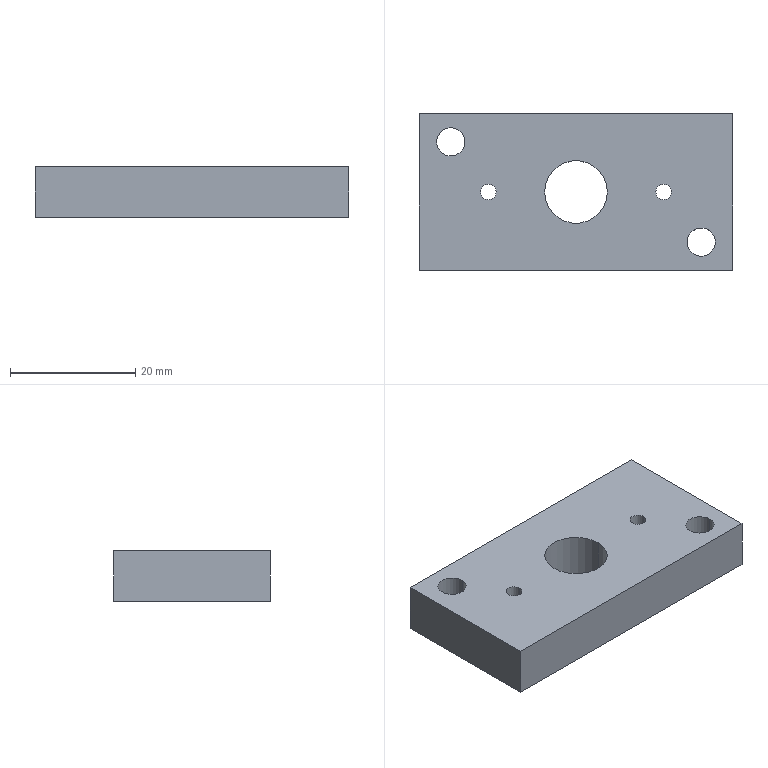Part | STEP file | positioning cylinder plate-1 | 1 solid | 16 faces | box 50 x 25 x 8 mm | volume 9039 mm3 | cylinder 10 | plane 6 | commonest cylinder face diameters 2.5 x4 4.5 x4 10 x2
STEP:
#1=CARTESIAN_POINT('',(0.,0.,0.));
#2=DIRECTION('',(0.,0.,1.));
#3=DIRECTION('',(1.,0.,0.));
#4=AXIS2_PLACEMENT_3D('',#1,#2,#3);
#5=CARTESIAN_POINT('',(-12.75,0.,0.));
#6=VERTEX_POINT('',#5);
#7=CARTESIAN_POINT('',(-12.75,0.,8.));
#8=VERTEX_POINT('',#7);
#9=CARTESIAN_POINT('',(-12.75,0.,8.));
#10=DIRECTION('',(0.,0.,1.));
#11=VECTOR('',#10,1.);
#12=LINE('',#9,#11);
#13=CARTESIAN_POINT('',(-14.,0.,8.));
#14=DIRECTION('',(0.,0.,1.));
#15=DIRECTION('',(1.,0.,0.));
#16=AXIS2_PLACEMENT_3D('',#13,#14,#15);
#17=CYLINDRICAL_SURFACE('',#16,1.25);
#18=CARTESIAN_POINT('',(6.283,0.));
#19=DIRECTION('',(0.,1.));
#20=VECTOR('',#19,1.);
#21=LINE('',#18,#20);
#22=(GEOMETRIC_REPRESENTATION_CONTEXT(2)PARAMETRIC_REPRESENTATION_CONTEXT()REPRESENTATION_CONTEXT('',''));
#23=DEFINITIONAL_REPRESENTATION('',(#21),#22);
#24=PCURVE('',#17,#23);
#25=CARTESIAN_POINT('',(-14.,0.,8.));
#26=DIRECTION('',(0.,0.,1.));
#27=DIRECTION('',(1.,0.,0.));
#28=AXIS2_PLACEMENT_3D('',#25,#26,#27);
#29=CYLINDRICAL_SURFACE('',#28,1.25);
#30=CARTESIAN_POINT('',(0.,0.));
#31=DIRECTION('',(0.,1.));
#32=VECTOR('',#31,1.);
#33=LINE('',#30,#32);
#34=(GEOMETRIC_REPRESENTATION_CONTEXT(2)PARAMETRIC_REPRESENTATION_CONTEXT()REPRESENTATION_CONTEXT('',''));
#35=DEFINITIONAL_REPRESENTATION('',(#33),#34);
#36=PCURVE('',#29,#35);
#37=SURFACE_CURVE('',#12,(#24,#36),.PCURVE_S1.);
#38=EDGE_CURVE('',#6,#8,#37,.T.);
#39=ORIENTED_EDGE('',*,*,#38,.T.);
#40=CARTESIAN_POINT('',(-15.25,0.,8.));
#41=VERTEX_POINT('',#40);
#42=CARTESIAN_POINT('',(-14.,0.,8.));
#43=DIRECTION('',(0.,0.,1.));
#44=DIRECTION('',(1.,0.,0.));
#45=AXIS2_PLACEMENT_3D('',#42,#43,#44);
#46=CIRCLE('',#45,1.25);
#47=CARTESIAN_POINT('',(0.,0.));
#48=DIRECTION('',(1.,0.));
#49=VECTOR('',#48,1.);
#50=LINE('',#47,#49);
#51=(GEOMETRIC_REPRESENTATION_CONTEXT(2)PARAMETRIC_REPRESENTATION_CONTEXT()REPRESENTATION_CONTEXT('',''));
#52=DEFINITIONAL_REPRESENTATION('',(#50),#51);
#53=PCURVE('',#17,#52);
#54=CARTESIAN_POINT('',(25.,-12.5,8.));
#55=DIRECTION('',(0.,0.,1.));
#56=DIRECTION('',(1.,0.,0.));
#57=AXIS2_PLACEMENT_3D('',#54,#55,#56);
#58=PLANE('',#57);
#59=CARTESIAN_POINT('',(-39.,12.5));
#60=DIRECTION('',(1.,0.));
#61=AXIS2_PLACEMENT_2D('',#59,#60);
#62=CIRCLE('',#61,1.25);
#63=(GEOMETRIC_REPRESENTATION_CONTEXT(2)PARAMETRIC_REPRESENTATION_CONTEXT()REPRESENTATION_CONTEXT('',''));
#64=DEFINITIONAL_REPRESENTATION('',(#62),#63);
#65=PCURVE('',#58,#64);
#66=SURFACE_CURVE('',#46,(#53,#65),.PCURVE_S1.);
#67=EDGE_CURVE('',#41,#8,#66,.T.);
#68=ORIENTED_EDGE('',*,*,#67,.F.);
#69=CARTESIAN_POINT('',(-15.25,0.,0.));
#70=VERTEX_POINT('',#69);
#71=CARTESIAN_POINT('',(-15.25,0.,8.));
#72=DIRECTION('',(0.,0.,1.));
#73=VECTOR('',#72,1.);
#74=LINE('',#71,#73);
#75=CARTESIAN_POINT('',(3.142,0.));
#76=DIRECTION('',(0.,1.));
#77=VECTOR('',#76,1.);
#78=LINE('',#75,#77);
#79=(GEOMETRIC_REPRESENTATION_CONTEXT(2)PARAMETRIC_REPRESENTATION_CONTEXT()REPRESENTATION_CONTEXT('',''));
#80=DEFINITIONAL_REPRESENTATION('',(#78),#79);
#81=PCURVE('',#17,#80);
#82=CARTESIAN_POINT('',(3.142,0.));
#83=DIRECTION('',(0.,1.));
#84=VECTOR('',#83,1.);
#85=LINE('',#82,#84);
#86=(GEOMETRIC_REPRESENTATION_CONTEXT(2)PARAMETRIC_REPRESENTATION_CONTEXT()REPRESENTATION_CONTEXT('',''));
#87=DEFINITIONAL_REPRESENTATION('',(#85),#86);
#88=PCURVE('',#29,#87);
#89=SURFACE_CURVE('',#74,(#81,#88),.PCURVE_S1.);
#90=EDGE_CURVE('',#70,#41,#89,.T.);
#91=ORIENTED_EDGE('',*,*,#90,.F.);
#92=CARTESIAN_POINT('',(-14.,0.,0.));
#93=DIRECTION('',(0.,0.,1.));
#94=DIRECTION('',(1.,0.,0.));
#95=AXIS2_PLACEMENT_3D('',#92,#93,#94);
#96=CIRCLE('',#95,1.25);
#97=CARTESIAN_POINT('',(0.,-8.));
#98=DIRECTION('',(1.,0.));
#99=VECTOR('',#98,1.);
#100=LINE('',#97,#99);
#101=(GEOMETRIC_REPRESENTATION_CONTEXT(2)PARAMETRIC_REPRESENTATION_CONTEXT()REPRESENTATION_CONTEXT('',''));
#102=DEFINITIONAL_REPRESENTATION('',(#100),#101);
#103=PCURVE('',#17,#102);
#104=CARTESIAN_POINT('',(25.,-12.5,0.));
#105=DIRECTION('',(0.,0.,1.));
#106=DIRECTION('',(1.,0.,0.));
#107=AXIS2_PLACEMENT_3D('',#104,#105,#106);
#108=PLANE('',#107);
#109=CARTESIAN_POINT('',(-39.,12.5));
#110=DIRECTION('',(1.,0.));
#111=AXIS2_PLACEMENT_2D('',#109,#110);
#112=CIRCLE('',#111,1.25);
#113=(GEOMETRIC_REPRESENTATION_CONTEXT(2)PARAMETRIC_REPRESENTATION_CONTEXT()REPRESENTATION_CONTEXT('',''));
#114=DEFINITIONAL_REPRESENTATION('',(#112),#113);
#115=PCURVE('',#108,#114);
#116=SURFACE_CURVE('',#96,(#103,#115),.PCURVE_S1.);
#117=EDGE_CURVE('',#70,#6,#116,.T.);
#118=ORIENTED_EDGE('',*,*,#117,.T.);
#119=EDGE_LOOP('',(#39,#68,#91,#118));
#120=FACE_BOUND('',#119,.F.);
#121=ADVANCED_FACE('',(#120),#17,.F.);
#122=CARTESIAN_POINT('',(15.25,0.,0.));
#123=VERTEX_POINT('',#122);
#124=CARTESIAN_POINT('',(15.25,0.,8.));
#125=VERTEX_POINT('',#124);
#126=CARTESIAN_POINT('',(15.25,0.,8.));
#127=DIRECTION('',(0.,0.,1.));
#128=VECTOR('',#127,1.);
#129=LINE('',#126,#128);
#130=CARTESIAN_POINT('',(14.,0.,8.));
#131=DIRECTION('',(0.,0.,1.));
#132=DIRECTION('',(1.,0.,0.));
#133=AXIS2_PLACEMENT_3D('',#130,#131,#132);
#134=CYLINDRICAL_SURFACE('',#133,1.25);
#135=CARTESIAN_POINT('',(6.283,0.));
#136=DIRECTION('',(0.,1.));
#137=VECTOR('',#136,1.);
#138=LINE('',#135,#137);
#139=(GEOMETRIC_REPRESENTATION_CONTEXT(2)PARAMETRIC_REPRESENTATION_CONTEXT()REPRESENTATION_CONTEXT('',''));
#140=DEFINITIONAL_REPRESENTATION('',(#138),#139);
#141=PCURVE('',#134,#140);
#142=CARTESIAN_POINT('',(14.,0.,8.));
#143=DIRECTION('',(0.,0.,1.));
#144=DIRECTION('',(1.,0.,0.));
#145=AXIS2_PLACEMENT_3D('',#142,#143,#144);
#146=CYLINDRICAL_SURFACE('',#145,1.25);
#147=CARTESIAN_POINT('',(0.,0.));
#148=DIRECTION('',(0.,1.));
#149=VECTOR('',#148,1.);
#150=LINE('',#147,#149);
#151=(GEOMETRIC_REPRESENTATION_CONTEXT(2)PARAMETRIC_REPRESENTATION_CONTEXT()REPRESENTATION_CONTEXT('',''));
#152=DEFINITIONAL_REPRESENTATION('',(#150),#151);
#153=PCURVE('',#146,#152);
#154=SURFACE_CURVE('',#129,(#141,#153),.PCURVE_S1.);
#155=EDGE_CURVE('',#123,#125,#154,.T.);
#156=ORIENTED_EDGE('',*,*,#155,.T.);
#157=CARTESIAN_POINT('',(12.75,0.,8.));
#158=VERTEX_POINT('',#157);
#159=CARTESIAN_POINT('',(14.,0.,8.));
#160=DIRECTION('',(0.,0.,1.));
#161=DIRECTION('',(1.,0.,0.));
#162=AXIS2_PLACEMENT_3D('',#159,#160,#161);
#163=CIRCLE('',#162,1.25);
#164=CARTESIAN_POINT('',(0.,0.));
#165=DIRECTION('',(1.,0.));
#166=VECTOR('',#165,1.);
#167=LINE('',#164,#166);
#168=(GEOMETRIC_REPRESENTATION_CONTEXT(2)PARAMETRIC_REPRESENTATION_CONTEXT()REPRESENTATION_CONTEXT('',''));
#169=DEFINITIONAL_REPRESENTATION('',(#167),#168);
#170=PCURVE('',#134,#169);
#171=CARTESIAN_POINT('',(-11.,12.5));
#172=DIRECTION('',(1.,0.));
#173=AXIS2_PLACEMENT_2D('',#171,#172);
#174=CIRCLE('',#173,1.25);
#175=(GEOMETRIC_REPRESENTATION_CONTEXT(2)PARAMETRIC_REPRESENTATION_CONTEXT()REPRESENTATION_CONTEXT('',''));
#176=DEFINITIONAL_REPRESENTATION('',(#174),#175);
#177=PCURVE('',#58,#176);
#178=SURFACE_CURVE('',#163,(#170,#177),.PCURVE_S1.);
#179=EDGE_CURVE('',#158,#125,#178,.T.);
#180=ORIENTED_EDGE('',*,*,#179,.F.);
#181=CARTESIAN_POINT('',(12.75,0.,0.));
#182=VERTEX_POINT('',#181);
#183=CARTESIAN_POINT('',(12.75,0.,8.));
#184=DIRECTION('',(0.,0.,1.));
#185=VECTOR('',#184,1.);
#186=LINE('',#183,#185);
#187=CARTESIAN_POINT('',(3.142,0.));
#188=DIRECTION('',(0.,1.));
#189=VECTOR('',#188,1.);
#190=LINE('',#187,#189);
#191=(GEOMETRIC_REPRESENTATION_CONTEXT(2)PARAMETRIC_REPRESENTATION_CONTEXT()REPRESENTATION_CONTEXT('',''));
#192=DEFINITIONAL_REPRESENTATION('',(#190),#191);
#193=PCURVE('',#134,#192);
#194=CARTESIAN_POINT('',(3.142,0.));
#195=DIRECTION('',(0.,1.));
#196=VECTOR('',#195,1.);
#197=LINE('',#194,#196);
#198=(GEOMETRIC_REPRESENTATION_CONTEXT(2)PARAMETRIC_REPRESENTATION_CONTEXT()REPRESENTATION_CONTEXT('',''));
#199=DEFINITIONAL_REPRESENTATION('',(#197),#198);
#200=PCURVE('',#146,#199);
#201=SURFACE_CURVE('',#186,(#193,#200),.PCURVE_S1.);
#202=EDGE_CURVE('',#182,#158,#201,.T.);
#203=ORIENTED_EDGE('',*,*,#202,.F.);
#204=CARTESIAN_POINT('',(14.,0.,0.));
#205=DIRECTION('',(0.,0.,1.));
#206=DIRECTION('',(1.,0.,0.));
#207=AXIS2_PLACEMENT_3D('',#204,#205,#206);
#208=CIRCLE('',#207,1.25);
#209=CARTESIAN_POINT('',(0.,-8.));
#210=DIRECTION('',(1.,0.));
#211=VECTOR('',#210,1.);
#212=LINE('',#209,#211);
#213=(GEOMETRIC_REPRESENTATION_CONTEXT(2)PARAMETRIC_REPRESENTATION_CONTEXT()REPRESENTATION_CONTEXT('',''));
#214=DEFINITIONAL_REPRESENTATION('',(#212),#213);
#215=PCURVE('',#134,#214);
#216=CARTESIAN_POINT('',(-11.,12.5));
#217=DIRECTION('',(1.,0.));
#218=AXIS2_PLACEMENT_2D('',#216,#217);
#219=CIRCLE('',#218,1.25);
#220=(GEOMETRIC_REPRESENTATION_CONTEXT(2)PARAMETRIC_REPRESENTATION_CONTEXT()REPRESENTATION_CONTEXT('',''));
#221=DEFINITIONAL_REPRESENTATION('',(#219),#220);
#222=PCURVE('',#108,#221);
#223=SURFACE_CURVE('',#208,(#215,#222),.PCURVE_S1.);
#224=EDGE_CURVE('',#182,#123,#223,.T.);
#225=ORIENTED_EDGE('',*,*,#224,.T.);
#226=EDGE_LOOP('',(#156,#180,#203,#225));
#227=FACE_BOUND('',#226,.F.);
#228=ADVANCED_FACE('',(#227),#134,.F.);
#229=CARTESIAN_POINT('',(-5.,0.,8.));
#230=VERTEX_POINT('',#229);
#231=CARTESIAN_POINT('',(-5.,0.,0.));
#232=VERTEX_POINT('',#231);
#233=CARTESIAN_POINT('',(-5.,0.,8.));
#234=DIRECTION('',(0.,0.,-1.));
#235=VECTOR('',#234,1.);
#236=LINE('',#233,#235);
#237=CARTESIAN_POINT('',(0.,0.,8.));
#238=DIRECTION('',(0.,0.,-1.));
#239=DIRECTION('',(-1.,0.,0.));
#240=AXIS2_PLACEMENT_3D('',#237,#238,#239);
#241=CYLINDRICAL_SURFACE('',#240,5.);
#242=CARTESIAN_POINT('',(6.283,0.));
#243=DIRECTION('',(0.,1.));
#244=VECTOR('',#243,1.);
#245=LINE('',#242,#244);
#246=(GEOMETRIC_REPRESENTATION_CONTEXT(2)PARAMETRIC_REPRESENTATION_CONTEXT()REPRESENTATION_CONTEXT('',''));
#247=DEFINITIONAL_REPRESENTATION('',(#245),#246);
#248=PCURVE('',#241,#247);
#249=CARTESIAN_POINT('',(0.,0.,8.));
#250=DIRECTION('',(0.,0.,-1.));
#251=DIRECTION('',(-1.,0.,0.));
#252=AXIS2_PLACEMENT_3D('',#249,#250,#251);
#253=CYLINDRICAL_SURFACE('',#252,5.);
#254=CARTESIAN_POINT('',(0.,0.));
#255=DIRECTION('',(0.,1.));
#256=VECTOR('',#255,1.);
#257=LINE('',#254,#256);
#258=(GEOMETRIC_REPRESENTATION_CONTEXT(2)PARAMETRIC_REPRESENTATION_CONTEXT()REPRESENTATION_CONTEXT('',''));
#259=DEFINITIONAL_REPRESENTATION('',(#257),#258);
#260=PCURVE('',#253,#259);
#261=SURFACE_CURVE('',#236,(#248,#260),.PCURVE_S1.);
#262=EDGE_CURVE('',#230,#232,#261,.T.);
#263=ORIENTED_EDGE('',*,*,#262,.T.);
#264=CARTESIAN_POINT('',(5.,0.,0.));
#265=VERTEX_POINT('',#264);
#266=CARTESIAN_POINT('',(0.,0.,0.));
#267=DIRECTION('',(0.,0.,1.));
#268=DIRECTION('',(1.,0.,0.));
#269=AXIS2_PLACEMENT_3D('',#266,#267,#268);
#270=CIRCLE('',#269,5.);
#271=CARTESIAN_POINT('',(9.425,8.));
#272=DIRECTION('',(-1.,0.));
#273=VECTOR('',#272,1.);
#274=LINE('',#271,#273);
#275=(GEOMETRIC_REPRESENTATION_CONTEXT(2)PARAMETRIC_REPRESENTATION_CONTEXT()REPRESENTATION_CONTEXT('',''));
#276=DEFINITIONAL_REPRESENTATION('',(#274),#275);
#277=PCURVE('',#241,#276);
#278=CARTESIAN_POINT('',(-25.,12.5));
#279=DIRECTION('',(1.,0.));
#280=AXIS2_PLACEMENT_2D('',#278,#279);
#281=CIRCLE('',#280,5.);
#282=(GEOMETRIC_REPRESENTATION_CONTEXT(2)PARAMETRIC_REPRESENTATION_CONTEXT()REPRESENTATION_CONTEXT('',''));
#283=DEFINITIONAL_REPRESENTATION('',(#281),#282);
#284=PCURVE('',#108,#283);
#285=SURFACE_CURVE('',#270,(#277,#284),.PCURVE_S1.);
#286=EDGE_CURVE('',#232,#265,#285,.T.);
#287=ORIENTED_EDGE('',*,*,#286,.T.);
#288=CARTESIAN_POINT('',(5.,0.,8.));
#289=VERTEX_POINT('',#288);
#290=CARTESIAN_POINT('',(5.,0.,8.));
#291=DIRECTION('',(0.,0.,-1.));
#292=VECTOR('',#291,1.);
#293=LINE('',#290,#292);
#294=CARTESIAN_POINT('',(3.142,0.));
#295=DIRECTION('',(0.,1.));
#296=VECTOR('',#295,1.);
#297=LINE('',#294,#296);
#298=(GEOMETRIC_REPRESENTATION_CONTEXT(2)PARAMETRIC_REPRESENTATION_CONTEXT()REPRESENTATION_CONTEXT('',''));
#299=DEFINITIONAL_REPRESENTATION('',(#297),#298);
#300=PCURVE('',#241,#299);
#301=CARTESIAN_POINT('',(3.142,0.));
#302=DIRECTION('',(0.,1.));
#303=VECTOR('',#302,1.);
#304=LINE('',#301,#303);
#305=(GEOMETRIC_REPRESENTATION_CONTEXT(2)PARAMETRIC_REPRESENTATION_CONTEXT()REPRESENTATION_CONTEXT('',''));
#306=DEFINITIONAL_REPRESENTATION('',(#304),#305);
#307=PCURVE('',#253,#306);
#308=SURFACE_CURVE('',#293,(#300,#307),.PCURVE_S1.);
#309=EDGE_CURVE('',#289,#265,#308,.T.);
#310=ORIENTED_EDGE('',*,*,#309,.F.);
#311=CARTESIAN_POINT('',(0.,0.,8.));
#312=DIRECTION('',(0.,0.,1.));
#313=DIRECTION('',(1.,0.,0.));
#314=AXIS2_PLACEMENT_3D('',#311,#312,#313);
#315=CIRCLE('',#314,5.);
#316=CARTESIAN_POINT('',(9.425,0.));
#317=DIRECTION('',(-1.,0.));
#318=VECTOR('',#317,1.);
#319=LINE('',#316,#318);
#320=(GEOMETRIC_REPRESENTATION_CONTEXT(2)PARAMETRIC_REPRESENTATION_CONTEXT()REPRESENTATION_CONTEXT('',''));
#321=DEFINITIONAL_REPRESENTATION('',(#319),#320);
#322=PCURVE('',#241,#321);
#323=CARTESIAN_POINT('',(-25.,12.5));
#324=DIRECTION('',(1.,0.));
#325=AXIS2_PLACEMENT_2D('',#323,#324);
#326=CIRCLE('',#325,5.);
#327=(GEOMETRIC_REPRESENTATION_CONTEXT(2)PARAMETRIC_REPRESENTATION_CONTEXT()REPRESENTATION_CONTEXT('',''));
#328=DEFINITIONAL_REPRESENTATION('',(#326),#327);
#329=PCURVE('',#58,#328);
#330=SURFACE_CURVE('',#315,(#322,#329),.PCURVE_S1.);
#331=EDGE_CURVE('',#230,#289,#330,.T.);
#332=ORIENTED_EDGE('',*,*,#331,.F.);
#333=EDGE_LOOP('',(#263,#287,#310,#332));
#334=FACE_BOUND('',#333,.F.);
#335=ADVANCED_FACE('',(#334),#241,.F.);
#336=CARTESIAN_POINT('',(-22.25,8.,8.));
#337=VERTEX_POINT('',#336);
#338=CARTESIAN_POINT('',(-22.25,8.,0.));
#339=VERTEX_POINT('',#338);
#340=CARTESIAN_POINT('',(-22.25,8.,8.));
#341=DIRECTION('',(0.,0.,-1.));
#342=VECTOR('',#341,1.);
#343=LINE('',#340,#342);
#344=CARTESIAN_POINT('',(-20.,8.,8.));
#345=DIRECTION('',(0.,0.,-1.));
#346=DIRECTION('',(-1.,0.,0.));
#347=AXIS2_PLACEMENT_3D('',#344,#345,#346);
#348=CYLINDRICAL_SURFACE('',#347,2.25);
#349=CARTESIAN_POINT('',(6.283,0.));
#350=DIRECTION('',(0.,1.));
#351=VECTOR('',#350,1.);
#352=LINE('',#349,#351);
#353=(GEOMETRIC_REPRESENTATION_CONTEXT(2)PARAMETRIC_REPRESENTATION_CONTEXT()REPRESENTATION_CONTEXT('',''));
#354=DEFINITIONAL_REPRESENTATION('',(#352),#353);
#355=PCURVE('',#348,#354);
#356=CARTESIAN_POINT('',(-20.,8.,8.));
#357=DIRECTION('',(0.,0.,-1.));
#358=DIRECTION('',(-1.,0.,0.));
#359=AXIS2_PLACEMENT_3D('',#356,#357,#358);
#360=CYLINDRICAL_SURFACE('',#359,2.25);
#361=CARTESIAN_POINT('',(0.,0.));
#362=DIRECTION('',(0.,1.));
#363=VECTOR('',#362,1.);
#364=LINE('',#361,#363);
#365=(GEOMETRIC_REPRESENTATION_CONTEXT(2)PARAMETRIC_REPRESENTATION_CONTEXT()REPRESENTATION_CONTEXT('',''));
#366=DEFINITIONAL_REPRESENTATION('',(#364),#365);
#367=PCURVE('',#360,#366);
#368=SURFACE_CURVE('',#343,(#355,#367),.PCURVE_S1.);
#369=EDGE_CURVE('',#337,#339,#368,.T.);
#370=ORIENTED_EDGE('',*,*,#369,.T.);
#371=CARTESIAN_POINT('',(-17.75,8.,0.));
#372=VERTEX_POINT('',#371);
#373=CARTESIAN_POINT('',(-20.,8.,0.));
#374=DIRECTION('',(0.,0.,1.));
#375=DIRECTION('',(1.,0.,0.));
#376=AXIS2_PLACEMENT_3D('',#373,#374,#375);
#377=CIRCLE('',#376,2.25);
#378=CARTESIAN_POINT('',(9.425,8.));
#379=DIRECTION('',(-1.,0.));
#380=VECTOR('',#379,1.);
#381=LINE('',#378,#380);
#382=(GEOMETRIC_REPRESENTATION_CONTEXT(2)PARAMETRIC_REPRESENTATION_CONTEXT()REPRESENTATION_CONTEXT('',''));
#383=DEFINITIONAL_REPRESENTATION('',(#381),#382);
#384=PCURVE('',#348,#383);
#385=CARTESIAN_POINT('',(-45.,20.5));
#386=DIRECTION('',(1.,0.));
#387=AXIS2_PLACEMENT_2D('',#385,#386);
#388=CIRCLE('',#387,2.25);
#389=(GEOMETRIC_REPRESENTATION_CONTEXT(2)PARAMETRIC_REPRESENTATION_CONTEXT()REPRESENTATION_CONTEXT('',''));
#390=DEFINITIONAL_REPRESENTATION('',(#388),#389);
#391=PCURVE('',#108,#390);
#392=SURFACE_CURVE('',#377,(#384,#391),.PCURVE_S1.);
#393=EDGE_CURVE('',#339,#372,#392,.T.);
#394=ORIENTED_EDGE('',*,*,#393,.T.);
#395=CARTESIAN_POINT('',(-17.75,8.,8.));
#396=VERTEX_POINT('',#395);
#397=CARTESIAN_POINT('',(-17.75,8.,8.));
#398=DIRECTION('',(0.,0.,-1.));
#399=VECTOR('',#398,1.);
#400=LINE('',#397,#399);
#401=CARTESIAN_POINT('',(3.142,0.));
#402=DIRECTION('',(0.,1.));
#403=VECTOR('',#402,1.);
#404=LINE('',#401,#403);
#405=(GEOMETRIC_REPRESENTATION_CONTEXT(2)PARAMETRIC_REPRESENTATION_CONTEXT()REPRESENTATION_CONTEXT('',''));
#406=DEFINITIONAL_REPRESENTATION('',(#404),#405);
#407=PCURVE('',#348,#406);
#408=CARTESIAN_POINT('',(3.142,0.));
#409=DIRECTION('',(0.,1.));
#410=VECTOR('',#409,1.);
#411=LINE('',#408,#410);
#412=(GEOMETRIC_REPRESENTATION_CONTEXT(2)PARAMETRIC_REPRESENTATION_CONTEXT()REPRESENTATION_CONTEXT('',''));
#413=DEFINITIONAL_REPRESENTATION('',(#411),#412);
#414=PCURVE('',#360,#413);
#415=SURFACE_CURVE('',#400,(#407,#414),.PCURVE_S1.);
#416=EDGE_CURVE('',#396,#372,#415,.T.);
#417=ORIENTED_EDGE('',*,*,#416,.F.);
#418=CARTESIAN_POINT('',(-20.,8.,8.));
#419=DIRECTION('',(0.,0.,1.));
#420=DIRECTION('',(1.,0.,0.));
#421=AXIS2_PLACEMENT_3D('',#418,#419,#420);
#422=CIRCLE('',#421,2.25);
#423=CARTESIAN_POINT('',(9.425,0.));
#424=DIRECTION('',(-1.,0.));
#425=VECTOR('',#424,1.);
#426=LINE('',#423,#425);
#427=(GEOMETRIC_REPRESENTATION_CONTEXT(2)PARAMETRIC_REPRESENTATION_CONTEXT()REPRESENTATION_CONTEXT('',''));
#428=DEFINITIONAL_REPRESENTATION('',(#426),#427);
#429=PCURVE('',#348,#428);
#430=CARTESIAN_POINT('',(-45.,20.5));
#431=DIRECTION('',(1.,0.));
#432=AXIS2_PLACEMENT_2D('',#430,#431);
#433=CIRCLE('',#432,2.25);
#434=(GEOMETRIC_REPRESENTATION_CONTEXT(2)PARAMETRIC_REPRESENTATION_CONTEXT()REPRESENTATION_CONTEXT('',''));
#435=DEFINITIONAL_REPRESENTATION('',(#433),#434);
#436=PCURVE('',#58,#435);
#437=SURFACE_CURVE('',#422,(#429,#436),.PCURVE_S1.);
#438=EDGE_CURVE('',#337,#396,#437,.T.);
#439=ORIENTED_EDGE('',*,*,#438,.F.);
#440=EDGE_LOOP('',(#370,#394,#417,#439));
#441=FACE_BOUND('',#440,.F.);
#442=ADVANCED_FACE('',(#441),#348,.F.);
#443=CARTESIAN_POINT('',(17.75,-8.,8.));
#444=VERTEX_POINT('',#443);
#445=CARTESIAN_POINT('',(17.75,-8.,0.));
#446=VERTEX_POINT('',#445);
#447=CARTESIAN_POINT('',(17.75,-8.,8.));
#448=DIRECTION('',(0.,0.,-1.));
#449=VECTOR('',#448,1.);
#450=LINE('',#447,#449);
#451=CARTESIAN_POINT('',(20.,-8.,8.));
#452=DIRECTION('',(0.,0.,-1.));
#453=DIRECTION('',(-1.,0.,0.));
#454=AXIS2_PLACEMENT_3D('',#451,#452,#453);
#455=CYLINDRICAL_SURFACE('',#454,2.25);
#456=CARTESIAN_POINT('',(6.283,0.));
#457=DIRECTION('',(0.,1.));
#458=VECTOR('',#457,1.);
#459=LINE('',#456,#458);
#460=(GEOMETRIC_REPRESENTATION_CONTEXT(2)PARAMETRIC_REPRESENTATION_CONTEXT()REPRESENTATION_CONTEXT('',''));
#461=DEFINITIONAL_REPRESENTATION('',(#459),#460);
#462=PCURVE('',#455,#461);
#463=CARTESIAN_POINT('',(20.,-8.,8.));
#464=DIRECTION('',(0.,0.,-1.));
#465=DIRECTION('',(-1.,0.,0.));
#466=AXIS2_PLACEMENT_3D('',#463,#464,#465);
#467=CYLINDRICAL_SURFACE('',#466,2.25);
#468=CARTESIAN_POINT('',(0.,0.));
#469=DIRECTION('',(0.,1.));
#470=VECTOR('',#469,1.);
#471=LINE('',#468,#470);
#472=(GEOMETRIC_REPRESENTATION_CONTEXT(2)PARAMETRIC_REPRESENTATION_CONTEXT()REPRESENTATION_CONTEXT('',''));
#473=DEFINITIONAL_REPRESENTATION('',(#471),#472);
#474=PCURVE('',#467,#473);
#475=SURFACE_CURVE('',#450,(#462,#474),.PCURVE_S1.);
#476=EDGE_CURVE('',#444,#446,#475,.T.);
#477=ORIENTED_EDGE('',*,*,#476,.T.);
#478=CARTESIAN_POINT('',(22.25,-8.,0.));
#479=VERTEX_POINT('',#478);
#480=CARTESIAN_POINT('',(20.,-8.,0.));
#481=DIRECTION('',(0.,0.,1.));
#482=DIRECTION('',(1.,0.,0.));
#483=AXIS2_PLACEMENT_3D('',#480,#481,#482);
#484=CIRCLE('',#483,2.25);
#485=CARTESIAN_POINT('',(9.425,8.));
#486=DIRECTION('',(-1.,0.));
#487=VECTOR('',#486,1.);
#488=LINE('',#485,#487);
#489=(GEOMETRIC_REPRESENTATION_CONTEXT(2)PARAMETRIC_REPRESENTATION_CONTEXT()REPRESENTATION_CONTEXT('',''));
#490=DEFINITIONAL_REPRESENTATION('',(#488),#489);
#491=PCURVE('',#455,#490);
#492=CARTESIAN_POINT('',(-5.,4.5));
#493=DIRECTION('',(1.,0.));
#494=AXIS2_PLACEMENT_2D('',#492,#493);
#495=CIRCLE('',#494,2.25);
#496=(GEOMETRIC_REPRESENTATION_CONTEXT(2)PARAMETRIC_REPRESENTATION_CONTEXT()REPRESENTATION_CONTEXT('',''));
#497=DEFINITIONAL_REPRESENTATION('',(#495),#496);
#498=PCURVE('',#108,#497);
#499=SURFACE_CURVE('',#484,(#491,#498),.PCURVE_S1.);
#500=EDGE_CURVE('',#446,#479,#499,.T.);
#501=ORIENTED_EDGE('',*,*,#500,.T.);
#502=CARTESIAN_POINT('',(22.25,-8.,8.));
#503=VERTEX_POINT('',#502);
#504=CARTESIAN_POINT('',(22.25,-8.,8.));
#505=DIRECTION('',(0.,0.,-1.));
#506=VECTOR('',#505,1.);
#507=LINE('',#504,#506);
#508=CARTESIAN_POINT('',(3.142,0.));
#509=DIRECTION('',(0.,1.));
#510=VECTOR('',#509,1.);
#511=LINE('',#508,#510);
#512=(GEOMETRIC_REPRESENTATION_CONTEXT(2)PARAMETRIC_REPRESENTATION_CONTEXT()REPRESENTATION_CONTEXT('',''));
#513=DEFINITIONAL_REPRESENTATION('',(#511),#512);
#514=PCURVE('',#455,#513);
#515=CARTESIAN_POINT('',(3.142,0.));
#516=DIRECTION('',(0.,1.));
#517=VECTOR('',#516,1.);
#518=LINE('',#515,#517);
#519=(GEOMETRIC_REPRESENTATION_CONTEXT(2)PARAMETRIC_REPRESENTATION_CONTEXT()REPRESENTATION_CONTEXT('',''));
#520=DEFINITIONAL_REPRESENTATION('',(#518),#519);
#521=PCURVE('',#467,#520);
#522=SURFACE_CURVE('',#507,(#514,#521),.PCURVE_S1.);
#523=EDGE_CURVE('',#503,#479,#522,.T.);
#524=ORIENTED_EDGE('',*,*,#523,.F.);
#525=CARTESIAN_POINT('',(20.,-8.,8.));
#526=DIRECTION('',(0.,0.,1.));
#527=DIRECTION('',(1.,0.,0.));
#528=AXIS2_PLACEMENT_3D('',#525,#526,#527);
#529=CIRCLE('',#528,2.25);
#530=CARTESIAN_POINT('',(9.425,0.));
#531=DIRECTION('',(-1.,0.));
#532=VECTOR('',#531,1.);
#533=LINE('',#530,#532);
#534=(GEOMETRIC_REPRESENTATION_CONTEXT(2)PARAMETRIC_REPRESENTATION_CONTEXT()REPRESENTATION_CONTEXT('',''));
#535=DEFINITIONAL_REPRESENTATION('',(#533),#534);
#536=PCURVE('',#455,#535);
#537=CARTESIAN_POINT('',(-5.,4.5));
#538=DIRECTION('',(1.,0.));
#539=AXIS2_PLACEMENT_2D('',#537,#538);
#540=CIRCLE('',#539,2.25);
#541=(GEOMETRIC_REPRESENTATION_CONTEXT(2)PARAMETRIC_REPRESENTATION_CONTEXT()REPRESENTATION_CONTEXT('',''));
#542=DEFINITIONAL_REPRESENTATION('',(#540),#541);
#543=PCURVE('',#58,#542);
#544=SURFACE_CURVE('',#529,(#536,#543),.PCURVE_S1.);
#545=EDGE_CURVE('',#444,#503,#544,.T.);
#546=ORIENTED_EDGE('',*,*,#545,.F.);
#547=EDGE_LOOP('',(#477,#501,#524,#546));
#548=FACE_BOUND('',#547,.F.);
#549=ADVANCED_FACE('',(#548),#455,.F.);
#550=CARTESIAN_POINT('',(-14.,0.,8.));
#551=DIRECTION('',(0.,0.,1.));
#552=DIRECTION('',(1.,0.,0.));
#553=AXIS2_PLACEMENT_3D('',#550,#551,#552);
#554=CIRCLE('',#553,1.25);
#555=CARTESIAN_POINT('',(-39.,12.5));
#556=DIRECTION('',(1.,0.));
#557=AXIS2_PLACEMENT_2D('',#555,#556);
#558=CIRCLE('',#557,1.25);
#559=(GEOMETRIC_REPRESENTATION_CONTEXT(2)PARAMETRIC_REPRESENTATION_CONTEXT()REPRESENTATION_CONTEXT('',''));
#560=DEFINITIONAL_REPRESENTATION('',(#558),#559);
#561=PCURVE('',#58,#560);
#562=CARTESIAN_POINT('',(0.,0.));
#563=DIRECTION('',(1.,0.));
#564=VECTOR('',#563,1.);
#565=LINE('',#562,#564);
#566=(GEOMETRIC_REPRESENTATION_CONTEXT(2)PARAMETRIC_REPRESENTATION_CONTEXT()REPRESENTATION_CONTEXT('',''));
#567=DEFINITIONAL_REPRESENTATION('',(#565),#566);
#568=PCURVE('',#29,#567);
#569=SURFACE_CURVE('',#554,(#561,#568),.PCURVE_S1.);
#570=EDGE_CURVE('',#8,#41,#569,.T.);
#571=ORIENTED_EDGE('',*,*,#570,.F.);
#572=ORIENTED_EDGE('',*,*,#67,.F.);
#573=EDGE_LOOP('',(#571,#572));
#574=FACE_BOUND('',#573,.T.);
#575=CARTESIAN_POINT('',(14.,0.,8.));
#576=DIRECTION('',(0.,0.,1.));
#577=DIRECTION('',(1.,0.,0.));
#578=AXIS2_PLACEMENT_3D('',#575,#576,#577);
#579=CIRCLE('',#578,1.25);
#580=CARTESIAN_POINT('',(-11.,12.5));
#581=DIRECTION('',(1.,0.));
#582=AXIS2_PLACEMENT_2D('',#580,#581);
#583=CIRCLE('',#582,1.25);
#584=(GEOMETRIC_REPRESENTATION_CONTEXT(2)PARAMETRIC_REPRESENTATION_CONTEXT()REPRESENTATION_CONTEXT('',''));
#585=DEFINITIONAL_REPRESENTATION('',(#583),#584);
#586=PCURVE('',#58,#585);
#587=CARTESIAN_POINT('',(0.,0.));
#588=DIRECTION('',(1.,0.));
#589=VECTOR('',#588,1.);
#590=LINE('',#587,#589);
#591=(GEOMETRIC_REPRESENTATION_CONTEXT(2)PARAMETRIC_REPRESENTATION_CONTEXT()REPRESENTATION_CONTEXT('',''));
#592=DEFINITIONAL_REPRESENTATION('',(#590),#591);
#593=PCURVE('',#146,#592);
#594=SURFACE_CURVE('',#579,(#586,#593),.PCURVE_S1.);
#595=EDGE_CURVE('',#125,#158,#594,.T.);
#596=ORIENTED_EDGE('',*,*,#595,.F.);
#597=ORIENTED_EDGE('',*,*,#179,.F.);
#598=EDGE_LOOP('',(#596,#597));
#599=FACE_BOUND('',#598,.T.);
#600=ORIENTED_EDGE('',*,*,#438,.F.);
#601=CARTESIAN_POINT('',(-20.,8.,8.));
#602=DIRECTION('',(0.,0.,1.));
#603=DIRECTION('',(1.,0.,0.));
#604=AXIS2_PLACEMENT_3D('',#601,#602,#603);
#605=CIRCLE('',#604,2.25);
#606=CARTESIAN_POINT('',(-45.,20.5));
#607=DIRECTION('',(1.,0.));
#608=AXIS2_PLACEMENT_2D('',#606,#607);
#609=CIRCLE('',#608,2.25);
#610=(GEOMETRIC_REPRESENTATION_CONTEXT(2)PARAMETRIC_REPRESENTATION_CONTEXT()REPRESENTATION_CONTEXT('',''));
#611=DEFINITIONAL_REPRESENTATION('',(#609),#610);
#612=PCURVE('',#58,#611);
#613=CARTESIAN_POINT('',(3.142,0.));
#614=DIRECTION('',(-1.,0.));
#615=VECTOR('',#614,1.);
#616=LINE('',#613,#615);
#617=(GEOMETRIC_REPRESENTATION_CONTEXT(2)PARAMETRIC_REPRESENTATION_CONTEXT()REPRESENTATION_CONTEXT('',''));
#618=DEFINITIONAL_REPRESENTATION('',(#616),#617);
#619=PCURVE('',#360,#618);
#620=SURFACE_CURVE('',#605,(#612,#619),.PCURVE_S1.);
#621=EDGE_CURVE('',#396,#337,#620,.T.);
#622=ORIENTED_EDGE('',*,*,#621,.F.);
#623=EDGE_LOOP('',(#600,#622));
#624=FACE_BOUND('',#623,.T.);
#625=CARTESIAN_POINT('',(25.,-12.5,8.));
#626=VERTEX_POINT('',#625);
#627=CARTESIAN_POINT('',(25.,12.5,8.));
#628=VERTEX_POINT('',#627);
#629=CARTESIAN_POINT('',(25.,12.5,8.));
#630=DIRECTION('',(0.,1.,0.));
#631=VECTOR('',#630,1.);
#632=LINE('',#629,#631);
#633=CARTESIAN_POINT('',(0.,25.));
#634=DIRECTION('',(0.,1.));
#635=VECTOR('',#634,1.);
#636=LINE('',#633,#635);
#637=(GEOMETRIC_REPRESENTATION_CONTEXT(2)PARAMETRIC_REPRESENTATION_CONTEXT()REPRESENTATION_CONTEXT('',''));
#638=DEFINITIONAL_REPRESENTATION('',(#636),#637);
#639=PCURVE('',#58,#638);
#640=CARTESIAN_POINT('',(25.,12.5,8.));
#641=DIRECTION('',(-1.,0.,0.));
#642=DIRECTION('',(0.,-1.,0.));
#643=AXIS2_PLACEMENT_3D('',#640,#641,#642);
#644=PLANE('',#643);
#645=CARTESIAN_POINT('',(0.,0.));
#646=DIRECTION('',(-1.,0.));
#647=VECTOR('',#646,1.);
#648=LINE('',#645,#647);
#649=(GEOMETRIC_REPRESENTATION_CONTEXT(2)PARAMETRIC_REPRESENTATION_CONTEXT()REPRESENTATION_CONTEXT('',''));
#650=DEFINITIONAL_REPRESENTATION('',(#648),#649);
#651=PCURVE('',#644,#650);
#652=SURFACE_CURVE('',#632,(#639,#651),.PCURVE_S1.);
#653=EDGE_CURVE('',#626,#628,#652,.T.);
#654=ORIENTED_EDGE('',*,*,#653,.T.);
#655=CARTESIAN_POINT('',(-25.,12.5,8.));
#656=VERTEX_POINT('',#655);
#657=CARTESIAN_POINT('',(-25.,12.5,8.));
#658=DIRECTION('',(-1.,0.,0.));
#659=VECTOR('',#658,1.);
#660=LINE('',#657,#659);
#661=CARTESIAN_POINT('',(-50.,25.));
#662=DIRECTION('',(-1.,0.));
#663=VECTOR('',#662,1.);
#664=LINE('',#661,#663);
#665=(GEOMETRIC_REPRESENTATION_CONTEXT(2)PARAMETRIC_REPRESENTATION_CONTEXT()REPRESENTATION_CONTEXT('',''));
#666=DEFINITIONAL_REPRESENTATION('',(#664),#665);
#667=PCURVE('',#58,#666);
#668=CARTESIAN_POINT('',(-25.,12.5,8.));
#669=DIRECTION('',(0.,-1.,0.));
#670=DIRECTION('',(0.,0.,-1.));
#671=AXIS2_PLACEMENT_3D('',#668,#669,#670);
#672=PLANE('',#671);
#673=CARTESIAN_POINT('',(0.,0.));
#674=DIRECTION('',(0.,-1.));
#675=VECTOR('',#674,1.);
#676=LINE('',#673,#675);
#677=(GEOMETRIC_REPRESENTATION_CONTEXT(2)PARAMETRIC_REPRESENTATION_CONTEXT()REPRESENTATION_CONTEXT('',''));
#678=DEFINITIONAL_REPRESENTATION('',(#676),#677);
#679=PCURVE('',#672,#678);
#680=SURFACE_CURVE('',#660,(#667,#679),.PCURVE_S1.);
#681=EDGE_CURVE('',#628,#656,#680,.T.);
#682=ORIENTED_EDGE('',*,*,#681,.T.);
#683=CARTESIAN_POINT('',(-25.,-12.5,8.));
#684=VERTEX_POINT('',#683);
#685=CARTESIAN_POINT('',(-25.,12.5,8.));
#686=DIRECTION('',(0.,-1.,0.));
#687=VECTOR('',#686,1.);
#688=LINE('',#685,#687);
#689=CARTESIAN_POINT('',(-50.,25.));
#690=DIRECTION('',(0.,-1.));
#691=VECTOR('',#690,1.);
#692=LINE('',#689,#691);
#693=(GEOMETRIC_REPRESENTATION_CONTEXT(2)PARAMETRIC_REPRESENTATION_CONTEXT()REPRESENTATION_CONTEXT('',''));
#694=DEFINITIONAL_REPRESENTATION('',(#692),#693);
#695=PCURVE('',#58,#694);
#696=CARTESIAN_POINT('',(-25.,12.5,8.));
#697=DIRECTION('',(1.,0.,0.));
#698=DIRECTION('',(0.,1.,0.));
#699=AXIS2_PLACEMENT_3D('',#696,#697,#698);
#700=PLANE('',#699);
#701=CARTESIAN_POINT('',(0.,0.));
#702=DIRECTION('',(-1.,0.));
#703=VECTOR('',#702,1.);
#704=LINE('',#701,#703);
#705=(GEOMETRIC_REPRESENTATION_CONTEXT(2)PARAMETRIC_REPRESENTATION_CONTEXT()REPRESENTATION_CONTEXT('',''));
#706=DEFINITIONAL_REPRESENTATION('',(#704),#705);
#707=PCURVE('',#700,#706);
#708=SURFACE_CURVE('',#688,(#695,#707),.PCURVE_S1.);
#709=EDGE_CURVE('',#656,#684,#708,.T.);
#710=ORIENTED_EDGE('',*,*,#709,.T.);
#711=CARTESIAN_POINT('',(-25.,-12.5,8.));
#712=DIRECTION('',(1.,0.,0.));
#713=VECTOR('',#712,1.);
#714=LINE('',#711,#713);
#715=CARTESIAN_POINT('',(-50.,0.));
#716=DIRECTION('',(1.,0.));
#717=VECTOR('',#716,1.);
#718=LINE('',#715,#717);
#719=(GEOMETRIC_REPRESENTATION_CONTEXT(2)PARAMETRIC_REPRESENTATION_CONTEXT()REPRESENTATION_CONTEXT('',''));
#720=DEFINITIONAL_REPRESENTATION('',(#718),#719);
#721=PCURVE('',#58,#720);
#722=CARTESIAN_POINT('',(-25.,-12.5,8.));
#723=DIRECTION('',(0.,1.,0.));
#724=DIRECTION('',(0.,0.,1.));
#725=AXIS2_PLACEMENT_3D('',#722,#723,#724);
#726=PLANE('',#725);
#727=CARTESIAN_POINT('',(0.,0.));
#728=DIRECTION('',(0.,1.));
#729=VECTOR('',#728,1.);
#730=LINE('',#727,#729);
#731=(GEOMETRIC_REPRESENTATION_CONTEXT(2)PARAMETRIC_REPRESENTATION_CONTEXT()REPRESENTATION_CONTEXT('',''));
#732=DEFINITIONAL_REPRESENTATION('',(#730),#731);
#733=PCURVE('',#726,#732);
#734=SURFACE_CURVE('',#714,(#721,#733),.PCURVE_S1.);
#735=EDGE_CURVE('',#684,#626,#734,.T.);
#736=ORIENTED_EDGE('',*,*,#735,.T.);
#737=EDGE_LOOP('',(#654,#682,#710,#736));
#738=FACE_BOUND('',#737,.T.);
#739=ORIENTED_EDGE('',*,*,#545,.F.);
#740=CARTESIAN_POINT('',(20.,-8.,8.));
#741=DIRECTION('',(0.,0.,1.));
#742=DIRECTION('',(1.,0.,0.));
#743=AXIS2_PLACEMENT_3D('',#740,#741,#742);
#744=CIRCLE('',#743,2.25);
#745=CARTESIAN_POINT('',(-5.,4.5));
#746=DIRECTION('',(1.,0.));
#747=AXIS2_PLACEMENT_2D('',#745,#746);
#748=CIRCLE('',#747,2.25);
#749=(GEOMETRIC_REPRESENTATION_CONTEXT(2)PARAMETRIC_REPRESENTATION_CONTEXT()REPRESENTATION_CONTEXT('',''));
#750=DEFINITIONAL_REPRESENTATION('',(#748),#749);
#751=PCURVE('',#58,#750);
#752=CARTESIAN_POINT('',(3.142,0.));
#753=DIRECTION('',(-1.,0.));
#754=VECTOR('',#753,1.);
#755=LINE('',#752,#754);
#756=(GEOMETRIC_REPRESENTATION_CONTEXT(2)PARAMETRIC_REPRESENTATION_CONTEXT()REPRESENTATION_CONTEXT('',''));
#757=DEFINITIONAL_REPRESENTATION('',(#755),#756);
#758=PCURVE('',#467,#757);
#759=SURFACE_CURVE('',#744,(#751,#758),.PCURVE_S1.);
#760=EDGE_CURVE('',#503,#444,#759,.T.);
#761=ORIENTED_EDGE('',*,*,#760,.F.);
#762=EDGE_LOOP('',(#739,#761));
#763=FACE_BOUND('',#762,.T.);
#764=ORIENTED_EDGE('',*,*,#331,.F.);
#765=CARTESIAN_POINT('',(0.,0.,8.));
#766=DIRECTION('',(0.,0.,1.));
#767=DIRECTION('',(1.,0.,0.));
#768=AXIS2_PLACEMENT_3D('',#765,#766,#767);
#769=CIRCLE('',#768,5.);
#770=CARTESIAN_POINT('',(-25.,12.5));
#771=DIRECTION('',(1.,0.));
#772=AXIS2_PLACEMENT_2D('',#770,#771);
#773=CIRCLE('',#772,5.);
#774=(GEOMETRIC_REPRESENTATION_CONTEXT(2)PARAMETRIC_REPRESENTATION_CONTEXT()REPRESENTATION_CONTEXT('',''));
#775=DEFINITIONAL_REPRESENTATION('',(#773),#774);
#776=PCURVE('',#58,#775);
#777=CARTESIAN_POINT('',(3.142,0.));
#778=DIRECTION('',(-1.,0.));
#779=VECTOR('',#778,1.);
#780=LINE('',#777,#779);
#781=(GEOMETRIC_REPRESENTATION_CONTEXT(2)PARAMETRIC_REPRESENTATION_CONTEXT()REPRESENTATION_CONTEXT('',''));
#782=DEFINITIONAL_REPRESENTATION('',(#780),#781);
#783=PCURVE('',#253,#782);
#784=SURFACE_CURVE('',#769,(#776,#783),.PCURVE_S1.);
#785=EDGE_CURVE('',#289,#230,#784,.T.);
#786=ORIENTED_EDGE('',*,*,#785,.F.);
#787=EDGE_LOOP('',(#764,#786));
#788=FACE_BOUND('',#787,.T.);
#789=ADVANCED_FACE('',(#574,#599,#624,#738,#763,#788),#58,.T.);
#790=CARTESIAN_POINT('',(-14.,0.,0.));
#791=DIRECTION('',(0.,0.,1.));
#792=DIRECTION('',(1.,0.,0.));
#793=AXIS2_PLACEMENT_3D('',#790,#791,#792);
#794=CIRCLE('',#793,1.25);
#795=CARTESIAN_POINT('',(-39.,12.5));
#796=DIRECTION('',(1.,0.));
#797=AXIS2_PLACEMENT_2D('',#795,#796);
#798=CIRCLE('',#797,1.25);
#799=(GEOMETRIC_REPRESENTATION_CONTEXT(2)PARAMETRIC_REPRESENTATION_CONTEXT()REPRESENTATION_CONTEXT('',''));
#800=DEFINITIONAL_REPRESENTATION('',(#798),#799);
#801=PCURVE('',#108,#800);
#802=CARTESIAN_POINT('',(0.,-8.));
#803=DIRECTION('',(1.,0.));
#804=VECTOR('',#803,1.);
#805=LINE('',#802,#804);
#806=(GEOMETRIC_REPRESENTATION_CONTEXT(2)PARAMETRIC_REPRESENTATION_CONTEXT()REPRESENTATION_CONTEXT('',''));
#807=DEFINITIONAL_REPRESENTATION('',(#805),#806);
#808=PCURVE('',#29,#807);
#809=SURFACE_CURVE('',#794,(#801,#808),.PCURVE_S1.);
#810=EDGE_CURVE('',#6,#70,#809,.T.);
#811=ORIENTED_EDGE('',*,*,#810,.T.);
#812=ORIENTED_EDGE('',*,*,#117,.T.);
#813=EDGE_LOOP('',(#811,#812));
#814=FACE_BOUND('',#813,.T.);
#815=CARTESIAN_POINT('',(14.,0.,0.));
#816=DIRECTION('',(0.,0.,1.));
#817=DIRECTION('',(1.,0.,0.));
#818=AXIS2_PLACEMENT_3D('',#815,#816,#817);
#819=CIRCLE('',#818,1.25);
#820=CARTESIAN_POINT('',(-11.,12.5));
#821=DIRECTION('',(1.,0.));
#822=AXIS2_PLACEMENT_2D('',#820,#821);
#823=CIRCLE('',#822,1.25);
#824=(GEOMETRIC_REPRESENTATION_CONTEXT(2)PARAMETRIC_REPRESENTATION_CONTEXT()REPRESENTATION_CONTEXT('',''));
#825=DEFINITIONAL_REPRESENTATION('',(#823),#824);
#826=PCURVE('',#108,#825);
#827=CARTESIAN_POINT('',(0.,-8.));
#828=DIRECTION('',(1.,0.));
#829=VECTOR('',#828,1.);
#830=LINE('',#827,#829);
#831=(GEOMETRIC_REPRESENTATION_CONTEXT(2)PARAMETRIC_REPRESENTATION_CONTEXT()REPRESENTATION_CONTEXT('',''));
#832=DEFINITIONAL_REPRESENTATION('',(#830),#831);
#833=PCURVE('',#146,#832);
#834=SURFACE_CURVE('',#819,(#826,#833),.PCURVE_S1.);
#835=EDGE_CURVE('',#123,#182,#834,.T.);
#836=ORIENTED_EDGE('',*,*,#835,.T.);
#837=ORIENTED_EDGE('',*,*,#224,.T.);
#838=EDGE_LOOP('',(#836,#837));
#839=FACE_BOUND('',#838,.T.);
#840=ORIENTED_EDGE('',*,*,#393,.T.);
#841=CARTESIAN_POINT('',(-20.,8.,0.));
#842=DIRECTION('',(0.,0.,1.));
#843=DIRECTION('',(1.,0.,0.));
#844=AXIS2_PLACEMENT_3D('',#841,#842,#843);
#845=CIRCLE('',#844,2.25);
#846=CARTESIAN_POINT('',(-45.,20.5));
#847=DIRECTION('',(1.,0.));
#848=AXIS2_PLACEMENT_2D('',#846,#847);
#849=CIRCLE('',#848,2.25);
#850=(GEOMETRIC_REPRESENTATION_CONTEXT(2)PARAMETRIC_REPRESENTATION_CONTEXT()REPRESENTATION_CONTEXT('',''));
#851=DEFINITIONAL_REPRESENTATION('',(#849),#850);
#852=PCURVE('',#108,#851);
#853=CARTESIAN_POINT('',(3.142,8.));
#854=DIRECTION('',(-1.,0.));
#855=VECTOR('',#854,1.);
#856=LINE('',#853,#855);
#857=(GEOMETRIC_REPRESENTATION_CONTEXT(2)PARAMETRIC_REPRESENTATION_CONTEXT()REPRESENTATION_CONTEXT('',''));
#858=DEFINITIONAL_REPRESENTATION('',(#856),#857);
#859=PCURVE('',#360,#858);
#860=SURFACE_CURVE('',#845,(#852,#859),.PCURVE_S1.);
#861=EDGE_CURVE('',#372,#339,#860,.T.);
#862=ORIENTED_EDGE('',*,*,#861,.T.);
#863=EDGE_LOOP('',(#840,#862));
#864=FACE_BOUND('',#863,.T.);
#865=CARTESIAN_POINT('',(25.,-12.5,0.));
#866=VERTEX_POINT('',#865);
#867=CARTESIAN_POINT('',(25.,12.5,0.));
#868=VERTEX_POINT('',#867);
#869=CARTESIAN_POINT('',(25.,12.5,0.));
#870=DIRECTION('',(0.,1.,0.));
#871=VECTOR('',#870,1.);
#872=LINE('',#869,#871);
#873=CARTESIAN_POINT('',(0.,25.));
#874=DIRECTION('',(0.,1.));
#875=VECTOR('',#874,1.);
#876=LINE('',#873,#875);
#877=(GEOMETRIC_REPRESENTATION_CONTEXT(2)PARAMETRIC_REPRESENTATION_CONTEXT()REPRESENTATION_CONTEXT('',''));
#878=DEFINITIONAL_REPRESENTATION('',(#876),#877);
#879=PCURVE('',#108,#878);
#880=CARTESIAN_POINT('',(0.,-8.));
#881=DIRECTION('',(-1.,0.));
#882=VECTOR('',#881,1.);
#883=LINE('',#880,#882);
#884=(GEOMETRIC_REPRESENTATION_CONTEXT(2)PARAMETRIC_REPRESENTATION_CONTEXT()REPRESENTATION_CONTEXT('',''));
#885=DEFINITIONAL_REPRESENTATION('',(#883),#884);
#886=PCURVE('',#644,#885);
#887=SURFACE_CURVE('',#872,(#879,#886),.PCURVE_S1.);
#888=EDGE_CURVE('',#866,#868,#887,.T.);
#889=ORIENTED_EDGE('',*,*,#888,.F.);
#890=CARTESIAN_POINT('',(-25.,-12.5,0.));
#891=VERTEX_POINT('',#890);
#892=CARTESIAN_POINT('',(-25.,-12.5,0.));
#893=DIRECTION('',(1.,0.,0.));
#894=VECTOR('',#893,1.);
#895=LINE('',#892,#894);
#896=CARTESIAN_POINT('',(-50.,0.));
#897=DIRECTION('',(1.,0.));
#898=VECTOR('',#897,1.);
#899=LINE('',#896,#898);
#900=(GEOMETRIC_REPRESENTATION_CONTEXT(2)PARAMETRIC_REPRESENTATION_CONTEXT()REPRESENTATION_CONTEXT('',''));
#901=DEFINITIONAL_REPRESENTATION('',(#899),#900);
#902=PCURVE('',#108,#901);
#903=CARTESIAN_POINT('',(-8.,0.));
#904=DIRECTION('',(0.,1.));
#905=VECTOR('',#904,1.);
#906=LINE('',#903,#905);
#907=(GEOMETRIC_REPRESENTATION_CONTEXT(2)PARAMETRIC_REPRESENTATION_CONTEXT()REPRESENTATION_CONTEXT('',''));
#908=DEFINITIONAL_REPRESENTATION('',(#906),#907);
#909=PCURVE('',#726,#908);
#910=SURFACE_CURVE('',#895,(#902,#909),.PCURVE_S1.);
#911=EDGE_CURVE('',#891,#866,#910,.T.);
#912=ORIENTED_EDGE('',*,*,#911,.F.);
#913=CARTESIAN_POINT('',(-25.,12.5,0.));
#914=VERTEX_POINT('',#913);
#915=CARTESIAN_POINT('',(-25.,12.5,0.));
#916=DIRECTION('',(0.,-1.,0.));
#917=VECTOR('',#916,1.);
#918=LINE('',#915,#917);
#919=CARTESIAN_POINT('',(-50.,25.));
#920=DIRECTION('',(0.,-1.));
#921=VECTOR('',#920,1.);
#922=LINE('',#919,#921);
#923=(GEOMETRIC_REPRESENTATION_CONTEXT(2)PARAMETRIC_REPRESENTATION_CONTEXT()REPRESENTATION_CONTEXT('',''));
#924=DEFINITIONAL_REPRESENTATION('',(#922),#923);
#925=PCURVE('',#108,#924);
#926=CARTESIAN_POINT('',(0.,-8.));
#927=DIRECTION('',(-1.,0.));
#928=VECTOR('',#927,1.);
#929=LINE('',#926,#928);
#930=(GEOMETRIC_REPRESENTATION_CONTEXT(2)PARAMETRIC_REPRESENTATION_CONTEXT()REPRESENTATION_CONTEXT('',''));
#931=DEFINITIONAL_REPRESENTATION('',(#929),#930);
#932=PCURVE('',#700,#931);
#933=SURFACE_CURVE('',#918,(#925,#932),.PCURVE_S1.);
#934=EDGE_CURVE('',#914,#891,#933,.T.);
#935=ORIENTED_EDGE('',*,*,#934,.F.);
#936=CARTESIAN_POINT('',(-25.,12.5,0.));
#937=DIRECTION('',(-1.,0.,0.));
#938=VECTOR('',#937,1.);
#939=LINE('',#936,#938);
#940=CARTESIAN_POINT('',(-50.,25.));
#941=DIRECTION('',(-1.,0.));
#942=VECTOR('',#941,1.);
#943=LINE('',#940,#942);
#944=(GEOMETRIC_REPRESENTATION_CONTEXT(2)PARAMETRIC_REPRESENTATION_CONTEXT()REPRESENTATION_CONTEXT('',''));
#945=DEFINITIONAL_REPRESENTATION('',(#943),#944);
#946=PCURVE('',#108,#945);
#947=CARTESIAN_POINT('',(8.,0.));
#948=DIRECTION('',(0.,-1.));
#949=VECTOR('',#948,1.);
#950=LINE('',#947,#949);
#951=(GEOMETRIC_REPRESENTATION_CONTEXT(2)PARAMETRIC_REPRESENTATION_CONTEXT()REPRESENTATION_CONTEXT('',''));
#952=DEFINITIONAL_REPRESENTATION('',(#950),#951);
#953=PCURVE('',#672,#952);
#954=SURFACE_CURVE('',#939,(#946,#953),.PCURVE_S1.);
#955=EDGE_CURVE('',#868,#914,#954,.T.);
#956=ORIENTED_EDGE('',*,*,#955,.F.);
#957=EDGE_LOOP('',(#889,#912,#935,#956));
#958=FACE_BOUND('',#957,.T.);
#959=ORIENTED_EDGE('',*,*,#500,.T.);
#960=CARTESIAN_POINT('',(20.,-8.,0.));
#961=DIRECTION('',(0.,0.,1.));
#962=DIRECTION('',(1.,0.,0.));
#963=AXIS2_PLACEMENT_3D('',#960,#961,#962);
#964=CIRCLE('',#963,2.25);
#965=CARTESIAN_POINT('',(-5.,4.5));
#966=DIRECTION('',(1.,0.));
#967=AXIS2_PLACEMENT_2D('',#965,#966);
#968=CIRCLE('',#967,2.25);
#969=(GEOMETRIC_REPRESENTATION_CONTEXT(2)PARAMETRIC_REPRESENTATION_CONTEXT()REPRESENTATION_CONTEXT('',''));
#970=DEFINITIONAL_REPRESENTATION('',(#968),#969);
#971=PCURVE('',#108,#970);
#972=CARTESIAN_POINT('',(3.142,8.));
#973=DIRECTION('',(-1.,0.));
#974=VECTOR('',#973,1.);
#975=LINE('',#972,#974);
#976=(GEOMETRIC_REPRESENTATION_CONTEXT(2)PARAMETRIC_REPRESENTATION_CONTEXT()REPRESENTATION_CONTEXT('',''));
#977=DEFINITIONAL_REPRESENTATION('',(#975),#976);
#978=PCURVE('',#467,#977);
#979=SURFACE_CURVE('',#964,(#971,#978),.PCURVE_S1.);
#980=EDGE_CURVE('',#479,#446,#979,.T.);
#981=ORIENTED_EDGE('',*,*,#980,.T.);
#982=EDGE_LOOP('',(#959,#981));
#983=FACE_BOUND('',#982,.T.);
#984=ORIENTED_EDGE('',*,*,#286,.T.);
#985=CARTESIAN_POINT('',(0.,0.,0.));
#986=DIRECTION('',(0.,0.,1.));
#987=DIRECTION('',(1.,0.,0.));
#988=AXIS2_PLACEMENT_3D('',#985,#986,#987);
#989=CIRCLE('',#988,5.);
#990=CARTESIAN_POINT('',(-25.,12.5));
#991=DIRECTION('',(1.,0.));
#992=AXIS2_PLACEMENT_2D('',#990,#991);
#993=CIRCLE('',#992,5.);
#994=(GEOMETRIC_REPRESENTATION_CONTEXT(2)PARAMETRIC_REPRESENTATION_CONTEXT()REPRESENTATION_CONTEXT('',''));
#995=DEFINITIONAL_REPRESENTATION('',(#993),#994);
#996=PCURVE('',#108,#995);
#997=CARTESIAN_POINT('',(3.142,8.));
#998=DIRECTION('',(-1.,0.));
#999=VECTOR('',#998,1.);
#1000=LINE('',#997,#999);
#1001=(GEOMETRIC_REPRESENTATION_CONTEXT(2)PARAMETRIC_REPRESENTATION_CONTEXT()REPRESENTATION_CONTEXT('',''));
#1002=DEFINITIONAL_REPRESENTATION('',(#1000),#1001);
#1003=PCURVE('',#253,#1002);
#1004=SURFACE_CURVE('',#989,(#996,#1003),.PCURVE_S1.);
#1005=EDGE_CURVE('',#265,#232,#1004,.T.);
#1006=ORIENTED_EDGE('',*,*,#1005,.T.);
#1007=EDGE_LOOP('',(#984,#1006));
#1008=FACE_BOUND('',#1007,.T.);
#1009=ADVANCED_FACE('',(#814,#839,#864,#958,#983,#1008),#108,.F.);
#1010=ORIENTED_EDGE('',*,*,#888,.T.);
#1011=CARTESIAN_POINT('',(25.,12.5,8.));
#1012=DIRECTION('',(0.,0.,-1.));
#1013=VECTOR('',#1012,1.);
#1014=LINE('',#1011,#1013);
#1015=CARTESIAN_POINT('',(0.,0.));
#1016=DIRECTION('',(0.,-1.));
#1017=VECTOR('',#1016,1.);
#1018=LINE('',#1015,#1017);
#1019=(GEOMETRIC_REPRESENTATION_CONTEXT(2)PARAMETRIC_REPRESENTATION_CONTEXT()REPRESENTATION_CONTEXT('',''));
#1020=DEFINITIONAL_REPRESENTATION('',(#1018),#1019);
#1021=PCURVE('',#644,#1020);
#1022=CARTESIAN_POINT('',(0.,50.));
#1023=DIRECTION('',(1.,0.));
#1024=VECTOR('',#1023,1.);
#1025=LINE('',#1022,#1024);
#1026=(GEOMETRIC_REPRESENTATION_CONTEXT(2)PARAMETRIC_REPRESENTATION_CONTEXT()REPRESENTATION_CONTEXT('',''));
#1027=DEFINITIONAL_REPRESENTATION('',(#1025),#1026);
#1028=PCURVE('',#672,#1027);
#1029=SURFACE_CURVE('',#1014,(#1021,#1028),.PCURVE_S1.);
#1030=EDGE_CURVE('',#628,#868,#1029,.T.);
#1031=ORIENTED_EDGE('',*,*,#1030,.F.);
#1032=ORIENTED_EDGE('',*,*,#653,.F.);
#1033=CARTESIAN_POINT('',(25.,-12.5,8.));
#1034=DIRECTION('',(0.,0.,-1.));
#1035=VECTOR('',#1034,1.);
#1036=LINE('',#1033,#1035);
#1037=CARTESIAN_POINT('',(25.,0.));
#1038=DIRECTION('',(0.,-1.));
#1039=VECTOR('',#1038,1.);
#1040=LINE('',#1037,#1039);
#1041=(GEOMETRIC_REPRESENTATION_CONTEXT(2)PARAMETRIC_REPRESENTATION_CONTEXT()REPRESENTATION_CONTEXT('',''));
#1042=DEFINITIONAL_REPRESENTATION('',(#1040),#1041);
#1043=PCURVE('',#644,#1042);
#1044=CARTESIAN_POINT('',(0.,50.));
#1045=DIRECTION('',(-1.,0.));
#1046=VECTOR('',#1045,1.);
#1047=LINE('',#1044,#1046);
#1048=(GEOMETRIC_REPRESENTATION_CONTEXT(2)PARAMETRIC_REPRESENTATION_CONTEXT()REPRESENTATION_CONTEXT('',''));
#1049=DEFINITIONAL_REPRESENTATION('',(#1047),#1048);
#1050=PCURVE('',#726,#1049);
#1051=SURFACE_CURVE('',#1036,(#1043,#1050),.PCURVE_S1.);
#1052=EDGE_CURVE('',#626,#866,#1051,.T.);
#1053=ORIENTED_EDGE('',*,*,#1052,.T.);
#1054=EDGE_LOOP('',(#1010,#1031,#1032,#1053));
#1055=FACE_BOUND('',#1054,.T.);
#1056=ADVANCED_FACE('',(#1055),#644,.F.);
#1057=ORIENTED_EDGE('',*,*,#955,.T.);
#1058=CARTESIAN_POINT('',(-25.,12.5,8.));
#1059=DIRECTION('',(0.,0.,-1.));
#1060=VECTOR('',#1059,1.);
#1061=LINE('',#1058,#1060);
#1062=CARTESIAN_POINT('',(0.,0.));
#1063=DIRECTION('',(1.,0.));
#1064=VECTOR('',#1063,1.);
#1065=LINE('',#1062,#1064);
#1066=(GEOMETRIC_REPRESENTATION_CONTEXT(2)PARAMETRIC_REPRESENTATION_CONTEXT()REPRESENTATION_CONTEXT('',''));
#1067=DEFINITIONAL_REPRESENTATION('',(#1065),#1066);
#1068=PCURVE('',#672,#1067);
#1069=CARTESIAN_POINT('',(0.,0.));
#1070=DIRECTION('',(0.,-1.));
#1071=VECTOR('',#1070,1.);
#1072=LINE('',#1069,#1071);
#1073=(GEOMETRIC_REPRESENTATION_CONTEXT(2)PARAMETRIC_REPRESENTATION_CONTEXT()REPRESENTATION_CONTEXT('',''));
#1074=DEFINITIONAL_REPRESENTATION('',(#1072),#1073);
#1075=PCURVE('',#700,#1074);
#1076=SURFACE_CURVE('',#1061,(#1068,#1075),.PCURVE_S1.);
#1077=EDGE_CURVE('',#656,#914,#1076,.T.);
#1078=ORIENTED_EDGE('',*,*,#1077,.F.);
#1079=ORIENTED_EDGE('',*,*,#681,.F.);
#1080=ORIENTED_EDGE('',*,*,#1030,.T.);
#1081=EDGE_LOOP('',(#1057,#1078,#1079,#1080));
#1082=FACE_BOUND('',#1081,.T.);
#1083=ADVANCED_FACE('',(#1082),#672,.F.);
#1084=ORIENTED_EDGE('',*,*,#934,.T.);
#1085=CARTESIAN_POINT('',(-25.,-12.5,8.));
#1086=DIRECTION('',(0.,0.,-1.));
#1087=VECTOR('',#1086,1.);
#1088=LINE('',#1085,#1087);
#1089=CARTESIAN_POINT('',(-25.,0.));
#1090=DIRECTION('',(0.,-1.));
#1091=VECTOR('',#1090,1.);
#1092=LINE('',#1089,#1091);
#1093=(GEOMETRIC_REPRESENTATION_CONTEXT(2)PARAMETRIC_REPRESENTATION_CONTEXT()REPRESENTATION_CONTEXT('',''));
#1094=DEFINITIONAL_REPRESENTATION('',(#1092),#1093);
#1095=PCURVE('',#700,#1094);
#1096=CARTESIAN_POINT('',(0.,0.));
#1097=DIRECTION('',(-1.,0.));
#1098=VECTOR('',#1097,1.);
#1099=LINE('',#1096,#1098);
#1100=(GEOMETRIC_REPRESENTATION_CONTEXT(2)PARAMETRIC_REPRESENTATION_CONTEXT()REPRESENTATION_CONTEXT('',''));
#1101=DEFINITIONAL_REPRESENTATION('',(#1099),#1100);
#1102=PCURVE('',#726,#1101);
#1103=SURFACE_CURVE('',#1088,(#1095,#1102),.PCURVE_S1.);
#1104=EDGE_CURVE('',#684,#891,#1103,.T.);
#1105=ORIENTED_EDGE('',*,*,#1104,.F.);
#1106=ORIENTED_EDGE('',*,*,#709,.F.);
#1107=ORIENTED_EDGE('',*,*,#1077,.T.);
#1108=EDGE_LOOP('',(#1084,#1105,#1106,#1107));
#1109=FACE_BOUND('',#1108,.T.);
#1110=ADVANCED_FACE('',(#1109),#700,.F.);
#1111=ORIENTED_EDGE('',*,*,#911,.T.);
#1112=ORIENTED_EDGE('',*,*,#1052,.F.);
#1113=ORIENTED_EDGE('',*,*,#735,.F.);
#1114=ORIENTED_EDGE('',*,*,#1104,.T.);
#1115=EDGE_LOOP('',(#1111,#1112,#1113,#1114));
#1116=FACE_BOUND('',#1115,.T.);
#1117=ADVANCED_FACE('',(#1116),#726,.F.);
#1118=ORIENTED_EDGE('',*,*,#980,.T.);
#1119=ORIENTED_EDGE('',*,*,#476,.F.);
#1120=ORIENTED_EDGE('',*,*,#760,.F.);
#1121=ORIENTED_EDGE('',*,*,#523,.T.);
#1122=EDGE_LOOP('',(#1118,#1119,#1120,#1121));
#1123=FACE_BOUND('',#1122,.F.);
#1124=ADVANCED_FACE('',(#1123),#467,.F.);
#1125=ORIENTED_EDGE('',*,*,#861,.T.);
#1126=ORIENTED_EDGE('',*,*,#369,.F.);
#1127=ORIENTED_EDGE('',*,*,#621,.F.);
#1128=ORIENTED_EDGE('',*,*,#416,.T.);
#1129=EDGE_LOOP('',(#1125,#1126,#1127,#1128));
#1130=FACE_BOUND('',#1129,.F.);
#1131=ADVANCED_FACE('',(#1130),#360,.F.);
#1132=ORIENTED_EDGE('',*,*,#1005,.T.);
#1133=ORIENTED_EDGE('',*,*,#262,.F.);
#1134=ORIENTED_EDGE('',*,*,#785,.F.);
#1135=ORIENTED_EDGE('',*,*,#309,.T.);
#1136=EDGE_LOOP('',(#1132,#1133,#1134,#1135));
#1137=FACE_BOUND('',#1136,.F.);
#1138=ADVANCED_FACE('',(#1137),#253,.F.);
#1139=ORIENTED_EDGE('',*,*,#595,.F.);
#1140=ORIENTED_EDGE('',*,*,#155,.F.);
#1141=ORIENTED_EDGE('',*,*,#835,.T.);
#1142=ORIENTED_EDGE('',*,*,#202,.T.);
#1143=EDGE_LOOP('',(#1139,#1140,#1141,#1142));
#1144=FACE_BOUND('',#1143,.F.);
#1145=ADVANCED_FACE('',(#1144),#146,.F.);
#1146=ORIENTED_EDGE('',*,*,#570,.F.);
#1147=ORIENTED_EDGE('',*,*,#38,.F.);
#1148=ORIENTED_EDGE('',*,*,#810,.T.);
#1149=ORIENTED_EDGE('',*,*,#90,.T.);
#1150=EDGE_LOOP('',(#1146,#1147,#1148,#1149));
#1151=FACE_BOUND('',#1150,.F.);
#1152=ADVANCED_FACE('',(#1151),#29,.F.);
#1153=CLOSED_SHELL('',(#121,#228,#335,#442,#549,#789,#1009,#1056,#1083,#1110,#1117,#1124,#1131,#1138,#1145,#1152));
#1154=MANIFOLD_SOLID_BREP('',#1153);
#1155=(LENGTH_UNIT()NAMED_UNIT(*)SI_UNIT(.MILLI.,.METRE.));
#1156=UNCERTAINTY_MEASURE_WITH_UNIT(LENGTH_MEASURE(0.0000001),#1155,'','');
#1157=(NAMED_UNIT(*)PLANE_ANGLE_UNIT()SI_UNIT($,.RADIAN.));
#1158=(NAMED_UNIT(*)SI_UNIT($,.STERADIAN.)SOLID_ANGLE_UNIT());
#1159=(GEOMETRIC_REPRESENTATION_CONTEXT(3)GLOBAL_UNCERTAINTY_ASSIGNED_CONTEXT((#1156))GLOBAL_UNIT_ASSIGNED_CONTEXT((#1155,#1157,#1158))REPRESENTATION_CONTEXT('',''));
#1160=ADVANCED_BREP_SHAPE_REPRESENTATION('',(#4,#1154),#1159);